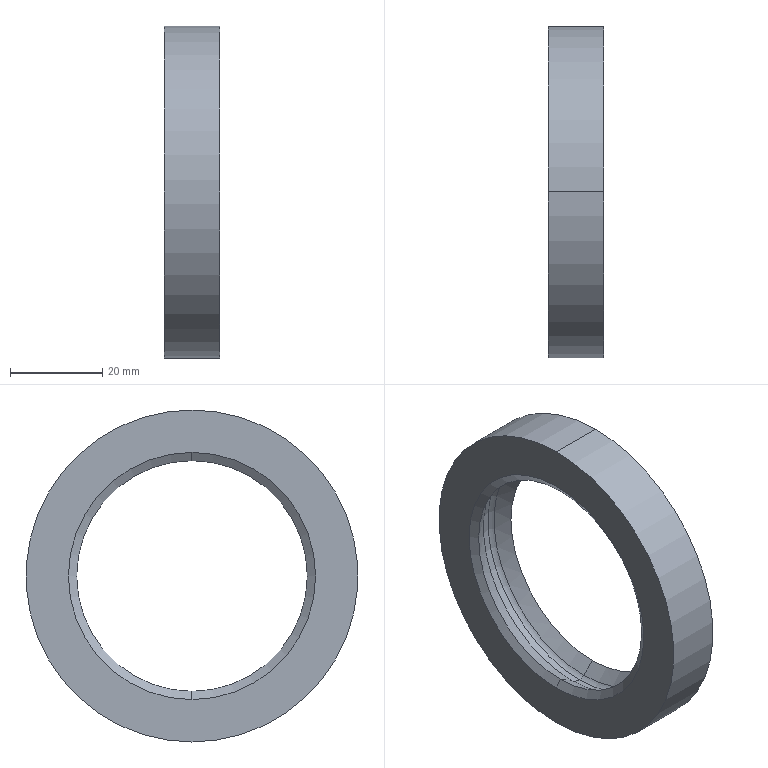Part | STEP file | AMFF-P5-A70-d50-D72-T12 oil seal | 1 solid | 17 faces | box 12 x 72 x 72 mm | volume 22091 mm3 | cone 10 | plane 3 | torus 2 | cylinder 2 | commonest cylinder face diameters 72 x2
STEP:
#1=CARTESIAN_POINT('',(0.,0.,0.));
#2=DIRECTION('',(0.,0.,1.));
#3=DIRECTION('',(1.,0.,0.));
#4=AXIS2_PLACEMENT_3D('',#1,#2,#3);
#5=CARTESIAN_POINT('',(-4.86,0.,25.));
#6=VERTEX_POINT('',#5);
#7=CARTESIAN_POINT('',(-6.,0.,26.8));
#8=VERTEX_POINT('',#7);
#9=CARTESIAN_POINT('',(-6.,0.,26.8));
#10=DIRECTION('',(-0.5351,0.,0.8448));
#11=VECTOR('',#10,1.);
#12=LINE('',#9,#11);
#13=CARTESIAN_POINT('',(-6.,0.,0.));
#14=DIRECTION('',(-1.,0.,0.));
#15=DIRECTION('',(0.,0.,1.));
#16=AXIS2_PLACEMENT_3D('',#13,#14,#15);
#17=CONICAL_SURFACE('',#16,26.8,1.006);
#18=CARTESIAN_POINT('',(6.283,0.));
#19=DIRECTION('',(0.,1.));
#20=VECTOR('',#19,1.);
#21=LINE('',#18,#20);
#22=(GEOMETRIC_REPRESENTATION_CONTEXT(2)PARAMETRIC_REPRESENTATION_CONTEXT()REPRESENTATION_CONTEXT('',''));
#23=DEFINITIONAL_REPRESENTATION('',(#21),#22);
#24=PCURVE('',#17,#23);
#25=CARTESIAN_POINT('',(-6.,0.,0.));
#26=DIRECTION('',(-1.,0.,0.));
#27=DIRECTION('',(0.,0.,1.));
#28=AXIS2_PLACEMENT_3D('',#25,#26,#27);
#29=CONICAL_SURFACE('',#28,26.8,1.006);
#30=CARTESIAN_POINT('',(0.,0.));
#31=DIRECTION('',(0.,1.));
#32=VECTOR('',#31,1.);
#33=LINE('',#30,#32);
#34=(GEOMETRIC_REPRESENTATION_CONTEXT(2)PARAMETRIC_REPRESENTATION_CONTEXT()REPRESENTATION_CONTEXT('',''));
#35=DEFINITIONAL_REPRESENTATION('',(#33),#34);
#36=PCURVE('',#29,#35);
#37=SURFACE_CURVE('',#12,(#24,#36),.PCURVE_S1.);
#38=EDGE_CURVE('',#6,#8,#37,.T.);
#39=ORIENTED_EDGE('',*,*,#38,.T.);
#40=CARTESIAN_POINT('',(-6.,0.,-26.8));
#41=VERTEX_POINT('',#40);
#42=CARTESIAN_POINT('',(-6.,0.,0.));
#43=DIRECTION('',(-1.,0.,0.));
#44=DIRECTION('',(0.,0.,1.));
#45=AXIS2_PLACEMENT_3D('',#42,#43,#44);
#46=CIRCLE('',#45,26.8);
#47=CARTESIAN_POINT('',(0.,0.));
#48=DIRECTION('',(1.,0.));
#49=VECTOR('',#48,1.);
#50=LINE('',#47,#49);
#51=(GEOMETRIC_REPRESENTATION_CONTEXT(2)PARAMETRIC_REPRESENTATION_CONTEXT()REPRESENTATION_CONTEXT('',''));
#52=DEFINITIONAL_REPRESENTATION('',(#50),#51);
#53=PCURVE('',#17,#52);
#54=CARTESIAN_POINT('',(-6.,26.8,0.));
#55=DIRECTION('',(1.,0.,0.));
#56=DIRECTION('',(0.,0.,-1.));
#57=AXIS2_PLACEMENT_3D('',#54,#55,#56);
#58=PLANE('',#57);
#59=CARTESIAN_POINT('',(-26.8,-26.8));
#60=CARTESIAN_POINT('',(-26.8,19.619));
#61=CARTESIAN_POINT('',(13.4,-3.591));
#62=CARTESIAN_POINT('',(53.6,-26.8));
#63=CARTESIAN_POINT('',(13.4,-50.009));
#64=CARTESIAN_POINT('',(-26.8,-73.219));
#65=CARTESIAN_POINT('',(-26.8,-26.8));
#66=(BOUNDED_CURVE()B_SPLINE_CURVE(2,(#59,#60,#61,#62,#63,#64,#65),.UNSPECIFIED.,.T.,.F.)B_SPLINE_CURVE_WITH_KNOTS((1,2,2,2,2,1),(-2.094,0.,2.094,4.189,6.283,8.378),.UNSPECIFIED.)CURVE()GEOMETRIC_REPRESENTATION_ITEM()RATIONAL_B_SPLINE_CURVE((1.,0.5,1.,0.5,1.,0.5,1.))REPRESENTATION_ITEM(''));
#67=(GEOMETRIC_REPRESENTATION_CONTEXT(2)PARAMETRIC_REPRESENTATION_CONTEXT()REPRESENTATION_CONTEXT('',''));
#68=DEFINITIONAL_REPRESENTATION('',(#66),#67);
#69=PCURVE('',#58,#68);
#70=SURFACE_CURVE('',#46,(#53,#69),.PCURVE_S1.);
#71=EDGE_CURVE('',#41,#8,#70,.T.);
#72=ORIENTED_EDGE('',*,*,#71,.F.);
#73=CARTESIAN_POINT('',(-4.86,0.,-25.));
#74=VERTEX_POINT('',#73);
#75=CARTESIAN_POINT('',(-6.,0.,-26.8));
#76=DIRECTION('',(-0.5351,0.,-0.8448));
#77=VECTOR('',#76,1.);
#78=LINE('',#75,#77);
#79=CARTESIAN_POINT('',(3.142,0.));
#80=DIRECTION('',(0.,1.));
#81=VECTOR('',#80,1.);
#82=LINE('',#79,#81);
#83=(GEOMETRIC_REPRESENTATION_CONTEXT(2)PARAMETRIC_REPRESENTATION_CONTEXT()REPRESENTATION_CONTEXT('',''));
#84=DEFINITIONAL_REPRESENTATION('',(#82),#83);
#85=PCURVE('',#17,#84);
#86=CARTESIAN_POINT('',(3.142,0.));
#87=DIRECTION('',(0.,1.));
#88=VECTOR('',#87,1.);
#89=LINE('',#86,#88);
#90=(GEOMETRIC_REPRESENTATION_CONTEXT(2)PARAMETRIC_REPRESENTATION_CONTEXT()REPRESENTATION_CONTEXT('',''));
#91=DEFINITIONAL_REPRESENTATION('',(#89),#90);
#92=PCURVE('',#29,#91);
#93=SURFACE_CURVE('',#78,(#85,#92),.PCURVE_S1.);
#94=EDGE_CURVE('',#74,#41,#93,.T.);
#95=ORIENTED_EDGE('',*,*,#94,.F.);
#96=CARTESIAN_POINT('',(-4.86,0.,0.));
#97=DIRECTION('',(-1.,0.,0.));
#98=DIRECTION('',(0.,0.,1.));
#99=AXIS2_PLACEMENT_3D('',#96,#97,#98);
#100=CIRCLE('',#99,25.);
#101=CARTESIAN_POINT('',(0.,-1.14));
#102=DIRECTION('',(1.,0.));
#103=VECTOR('',#102,1.);
#104=LINE('',#101,#103);
#105=(GEOMETRIC_REPRESENTATION_CONTEXT(2)PARAMETRIC_REPRESENTATION_CONTEXT()REPRESENTATION_CONTEXT('',''));
#106=DEFINITIONAL_REPRESENTATION('',(#104),#105);
#107=PCURVE('',#17,#106);
#108=CARTESIAN_POINT('',(-4.86,0.,0.));
#109=DIRECTION('',(1.,0.,0.));
#110=DIRECTION('',(0.,0.,-1.));
#111=AXIS2_PLACEMENT_3D('',#108,#109,#110);
#112=CONICAL_SURFACE('',#111,25.,0.5404);
#113=CARTESIAN_POINT('',(9.425,0.));
#114=DIRECTION('',(-1.,0.));
#115=VECTOR('',#114,1.);
#116=LINE('',#113,#115);
#117=(GEOMETRIC_REPRESENTATION_CONTEXT(2)PARAMETRIC_REPRESENTATION_CONTEXT()REPRESENTATION_CONTEXT('',''));
#118=DEFINITIONAL_REPRESENTATION('',(#116),#117);
#119=PCURVE('',#112,#118);
#120=SURFACE_CURVE('',#100,(#107,#119),.PCURVE_S1.);
#121=EDGE_CURVE('',#74,#6,#120,.T.);
#122=ORIENTED_EDGE('',*,*,#121,.T.);
#123=EDGE_LOOP('',(#39,#72,#95,#122));
#124=FACE_BOUND('',#123,.F.);
#125=ADVANCED_FACE('',(#124),#17,.F.);
#126=CARTESIAN_POINT('',(-1.26,0.,-27.16));
#127=VERTEX_POINT('',#126);
#128=CARTESIAN_POINT('',(-4.86,0.,-25.));
#129=DIRECTION('',(0.8575,0.,-0.5145));
#130=VECTOR('',#129,1.);
#131=LINE('',#128,#130);
#132=CARTESIAN_POINT('',(6.283,0.));
#133=DIRECTION('',(0.,1.));
#134=VECTOR('',#133,1.);
#135=LINE('',#132,#134);
#136=(GEOMETRIC_REPRESENTATION_CONTEXT(2)PARAMETRIC_REPRESENTATION_CONTEXT()REPRESENTATION_CONTEXT('',''));
#137=DEFINITIONAL_REPRESENTATION('',(#135),#136);
#138=PCURVE('',#112,#137);
#139=CARTESIAN_POINT('',(-4.86,0.,0.));
#140=DIRECTION('',(1.,0.,0.));
#141=DIRECTION('',(0.,0.,-1.));
#142=AXIS2_PLACEMENT_3D('',#139,#140,#141);
#143=CONICAL_SURFACE('',#142,25.,0.5404);
#144=CARTESIAN_POINT('',(0.,0.));
#145=DIRECTION('',(0.,1.));
#146=VECTOR('',#145,1.);
#147=LINE('',#144,#146);
#148=(GEOMETRIC_REPRESENTATION_CONTEXT(2)PARAMETRIC_REPRESENTATION_CONTEXT()REPRESENTATION_CONTEXT('',''));
#149=DEFINITIONAL_REPRESENTATION('',(#147),#148);
#150=PCURVE('',#143,#149);
#151=SURFACE_CURVE('',#131,(#138,#150),.PCURVE_S1.);
#152=EDGE_CURVE('',#74,#127,#151,.T.);
#153=ORIENTED_EDGE('',*,*,#152,.T.);
#154=CARTESIAN_POINT('',(-1.26,0.,27.16));
#155=VERTEX_POINT('',#154);
#156=CARTESIAN_POINT('',(-1.26,0.,0.));
#157=DIRECTION('',(-1.,0.,0.));
#158=DIRECTION('',(0.,0.,1.));
#159=AXIS2_PLACEMENT_3D('',#156,#157,#158);
#160=CIRCLE('',#159,27.16);
#161=CARTESIAN_POINT('',(9.425,3.6));
#162=DIRECTION('',(-1.,0.));
#163=VECTOR('',#162,1.);
#164=LINE('',#161,#163);
#165=(GEOMETRIC_REPRESENTATION_CONTEXT(2)PARAMETRIC_REPRESENTATION_CONTEXT()REPRESENTATION_CONTEXT('',''));
#166=DEFINITIONAL_REPRESENTATION('',(#164),#165);
#167=PCURVE('',#112,#166);
#168=CARTESIAN_POINT('',(-1.26,27.52,0.));
#169=DIRECTION('',(-1.,0.,0.));
#170=DIRECTION('',(0.,0.,1.));
#171=AXIS2_PLACEMENT_3D('',#168,#169,#170);
#172=PLANE('',#171);
#173=CARTESIAN_POINT('',(0.,-27.52));
#174=DIRECTION('',(1.,0.));
#175=AXIS2_PLACEMENT_2D('',#173,#174);
#176=CIRCLE('',#175,27.16);
#177=(GEOMETRIC_REPRESENTATION_CONTEXT(2)PARAMETRIC_REPRESENTATION_CONTEXT()REPRESENTATION_CONTEXT('',''));
#178=DEFINITIONAL_REPRESENTATION('',(#176),#177);
#179=PCURVE('',#172,#178);
#180=SURFACE_CURVE('',#160,(#167,#179),.PCURVE_S1.);
#181=EDGE_CURVE('',#127,#155,#180,.T.);
#182=ORIENTED_EDGE('',*,*,#181,.T.);
#183=CARTESIAN_POINT('',(-4.86,0.,25.));
#184=DIRECTION('',(0.8575,0.,0.5145));
#185=VECTOR('',#184,1.);
#186=LINE('',#183,#185);
#187=CARTESIAN_POINT('',(3.142,0.));
#188=DIRECTION('',(0.,1.));
#189=VECTOR('',#188,1.);
#190=LINE('',#187,#189);
#191=(GEOMETRIC_REPRESENTATION_CONTEXT(2)PARAMETRIC_REPRESENTATION_CONTEXT()REPRESENTATION_CONTEXT('',''));
#192=DEFINITIONAL_REPRESENTATION('',(#190),#191);
#193=PCURVE('',#112,#192);
#194=CARTESIAN_POINT('',(3.142,0.));
#195=DIRECTION('',(0.,1.));
#196=VECTOR('',#195,1.);
#197=LINE('',#194,#196);
#198=(GEOMETRIC_REPRESENTATION_CONTEXT(2)PARAMETRIC_REPRESENTATION_CONTEXT()REPRESENTATION_CONTEXT('',''));
#199=DEFINITIONAL_REPRESENTATION('',(#197),#198);
#200=PCURVE('',#143,#199);
#201=SURFACE_CURVE('',#186,(#193,#200),.PCURVE_S1.);
#202=EDGE_CURVE('',#6,#155,#201,.T.);
#203=ORIENTED_EDGE('',*,*,#202,.F.);
#204=ORIENTED_EDGE('',*,*,#121,.F.);
#205=EDGE_LOOP('',(#153,#182,#203,#204));
#206=FACE_BOUND('',#205,.F.);
#207=ADVANCED_FACE('',(#206),#112,.F.);
#208=CARTESIAN_POINT('',(-1.26,0.,-27.52));
#209=VERTEX_POINT('',#208);
#210=CARTESIAN_POINT('',(1.14,0.,-28.191));
#211=VERTEX_POINT('',#210);
#212=CARTESIAN_POINT('',(-1.26,0.,-27.52));
#213=DIRECTION('',(0.9631,0.,-0.2693));
#214=VECTOR('',#213,1.);
#215=LINE('',#212,#214);
#216=CARTESIAN_POINT('',(-1.26,0.,0.));
#217=DIRECTION('',(1.,0.,0.));
#218=DIRECTION('',(0.,0.,-1.));
#219=AXIS2_PLACEMENT_3D('',#216,#217,#218);
#220=CONICAL_SURFACE('',#219,27.52,0.2727);
#221=CARTESIAN_POINT('',(6.283,0.));
#222=DIRECTION('',(0.,1.));
#223=VECTOR('',#222,1.);
#224=LINE('',#221,#223);
#225=(GEOMETRIC_REPRESENTATION_CONTEXT(2)PARAMETRIC_REPRESENTATION_CONTEXT()REPRESENTATION_CONTEXT('',''));
#226=DEFINITIONAL_REPRESENTATION('',(#224),#225);
#227=PCURVE('',#220,#226);
#228=CARTESIAN_POINT('',(-1.26,0.,0.));
#229=DIRECTION('',(1.,0.,0.));
#230=DIRECTION('',(0.,0.,-1.));
#231=AXIS2_PLACEMENT_3D('',#228,#229,#230);
#232=CONICAL_SURFACE('',#231,27.52,0.2727);
#233=CARTESIAN_POINT('',(0.,0.));
#234=DIRECTION('',(0.,1.));
#235=VECTOR('',#234,1.);
#236=LINE('',#233,#235);
#237=(GEOMETRIC_REPRESENTATION_CONTEXT(2)PARAMETRIC_REPRESENTATION_CONTEXT()REPRESENTATION_CONTEXT('',''));
#238=DEFINITIONAL_REPRESENTATION('',(#236),#237);
#239=PCURVE('',#232,#238);
#240=SURFACE_CURVE('',#215,(#227,#239),.PCURVE_S1.);
#241=EDGE_CURVE('',#209,#211,#240,.T.);
#242=ORIENTED_EDGE('',*,*,#241,.T.);
#243=CARTESIAN_POINT('',(1.14,0.,28.191));
#244=VERTEX_POINT('',#243);
#245=CARTESIAN_POINT('',(1.14,0.,0.));
#246=DIRECTION('',(-1.,0.,0.));
#247=DIRECTION('',(0.,0.,1.));
#248=AXIS2_PLACEMENT_3D('',#245,#246,#247);
#249=CIRCLE('',#248,28.191);
#250=CARTESIAN_POINT('',(9.425,2.4));
#251=DIRECTION('',(-1.,0.));
#252=VECTOR('',#251,1.);
#253=LINE('',#250,#252);
#254=(GEOMETRIC_REPRESENTATION_CONTEXT(2)PARAMETRIC_REPRESENTATION_CONTEXT()REPRESENTATION_CONTEXT('',''));
#255=DEFINITIONAL_REPRESENTATION('',(#253),#254);
#256=PCURVE('',#220,#255);
#257=CARTESIAN_POINT('',(0.3749,0.,0.));
#258=DIRECTION('',(-1.,0.,0.));
#259=DIRECTION('',(0.,0.,1.));
#260=AXIS2_PLACEMENT_3D('',#257,#258,#259);
#261=TOROIDAL_SURFACE('',#260,25.415,2.88);
#262=CARTESIAN_POINT('',(0.,6.014));
#263=DIRECTION('',(1.,0.));
#264=VECTOR('',#263,1.);
#265=LINE('',#262,#264);
#266=(GEOMETRIC_REPRESENTATION_CONTEXT(2)PARAMETRIC_REPRESENTATION_CONTEXT()REPRESENTATION_CONTEXT('',''));
#267=DEFINITIONAL_REPRESENTATION('',(#265),#266);
#268=PCURVE('',#261,#267);
#269=SURFACE_CURVE('',#249,(#256,#268),.PCURVE_S1.);
#270=EDGE_CURVE('',#211,#244,#269,.T.);
#271=ORIENTED_EDGE('',*,*,#270,.T.);
#272=CARTESIAN_POINT('',(-1.26,0.,27.52));
#273=VERTEX_POINT('',#272);
#274=CARTESIAN_POINT('',(-1.26,0.,27.52));
#275=DIRECTION('',(0.9631,0.,0.2693));
#276=VECTOR('',#275,1.);
#277=LINE('',#274,#276);
#278=CARTESIAN_POINT('',(3.142,0.));
#279=DIRECTION('',(0.,1.));
#280=VECTOR('',#279,1.);
#281=LINE('',#278,#280);
#282=(GEOMETRIC_REPRESENTATION_CONTEXT(2)PARAMETRIC_REPRESENTATION_CONTEXT()REPRESENTATION_CONTEXT('',''));
#283=DEFINITIONAL_REPRESENTATION('',(#281),#282);
#284=PCURVE('',#220,#283);
#285=CARTESIAN_POINT('',(3.142,0.));
#286=DIRECTION('',(0.,1.));
#287=VECTOR('',#286,1.);
#288=LINE('',#285,#287);
#289=(GEOMETRIC_REPRESENTATION_CONTEXT(2)PARAMETRIC_REPRESENTATION_CONTEXT()REPRESENTATION_CONTEXT('',''));
#290=DEFINITIONAL_REPRESENTATION('',(#288),#289);
#291=PCURVE('',#232,#290);
#292=SURFACE_CURVE('',#277,(#284,#291),.PCURVE_S1.);
#293=EDGE_CURVE('',#273,#244,#292,.T.);
#294=ORIENTED_EDGE('',*,*,#293,.F.);
#295=CARTESIAN_POINT('',(-1.26,0.,0.));
#296=DIRECTION('',(-1.,0.,0.));
#297=DIRECTION('',(0.,0.,1.));
#298=AXIS2_PLACEMENT_3D('',#295,#296,#297);
#299=CIRCLE('',#298,27.52);
#300=CARTESIAN_POINT('',(9.425,0.));
#301=DIRECTION('',(-1.,0.));
#302=VECTOR('',#301,1.);
#303=LINE('',#300,#302);
#304=(GEOMETRIC_REPRESENTATION_CONTEXT(2)PARAMETRIC_REPRESENTATION_CONTEXT()REPRESENTATION_CONTEXT('',''));
#305=DEFINITIONAL_REPRESENTATION('',(#303),#304);
#306=PCURVE('',#220,#305);
#307=CARTESIAN_POINT('',(0.,-27.52));
#308=DIRECTION('',(1.,0.));
#309=AXIS2_PLACEMENT_2D('',#307,#308);
#310=CIRCLE('',#309,27.52);
#311=(GEOMETRIC_REPRESENTATION_CONTEXT(2)PARAMETRIC_REPRESENTATION_CONTEXT()REPRESENTATION_CONTEXT('',''));
#312=DEFINITIONAL_REPRESENTATION('',(#310),#311);
#313=PCURVE('',#172,#312);
#314=SURFACE_CURVE('',#299,(#306,#313),.PCURVE_S1.);
#315=EDGE_CURVE('',#209,#273,#314,.T.);
#316=ORIENTED_EDGE('',*,*,#315,.F.);
#317=EDGE_LOOP('',(#242,#271,#294,#316));
#318=FACE_BOUND('',#317,.F.);
#319=ADVANCED_FACE('',(#318),#220,.F.);
#320=CARTESIAN_POINT('',(2.34,0.,27.52));
#321=VERTEX_POINT('',#320);
#322=CARTESIAN_POINT('',(0.3749,0.,25.415));
#323=DIRECTION('',(0.,-1.,0.));
#324=DIRECTION('',(0.,0.,-1.));
#325=AXIS2_PLACEMENT_3D('',#322,#323,#324);
#326=CIRCLE('',#325,2.88);
#327=CARTESIAN_POINT('',(6.283,3.142));
#328=DIRECTION('',(0.,1.));
#329=VECTOR('',#328,1.);
#330=LINE('',#327,#329);
#331=(GEOMETRIC_REPRESENTATION_CONTEXT(2)PARAMETRIC_REPRESENTATION_CONTEXT()REPRESENTATION_CONTEXT('',''));
#332=DEFINITIONAL_REPRESENTATION('',(#330),#331);
#333=PCURVE('',#261,#332);
#334=CARTESIAN_POINT('',(0.3749,0.,0.));
#335=DIRECTION('',(-1.,0.,0.));
#336=DIRECTION('',(0.,0.,1.));
#337=AXIS2_PLACEMENT_3D('',#334,#335,#336);
#338=TOROIDAL_SURFACE('',#337,25.415,2.88);
#339=CARTESIAN_POINT('',(0.,3.142));
#340=DIRECTION('',(0.,1.));
#341=VECTOR('',#340,1.);
#342=LINE('',#339,#341);
#343=(GEOMETRIC_REPRESENTATION_CONTEXT(2)PARAMETRIC_REPRESENTATION_CONTEXT()REPRESENTATION_CONTEXT('',''));
#344=DEFINITIONAL_REPRESENTATION('',(#342),#343);
#345=PCURVE('',#338,#344);
#346=SURFACE_CURVE('',#326,(#333,#345),.PCURVE_S1.);
#347=EDGE_CURVE('',#321,#244,#346,.T.);
#348=ORIENTED_EDGE('',*,*,#347,.T.);
#349=ORIENTED_EDGE('',*,*,#270,.F.);
#350=CARTESIAN_POINT('',(2.34,0.,-27.52));
#351=VERTEX_POINT('',#350);
#352=CARTESIAN_POINT('',(0.3749,0.,-25.415));
#353=DIRECTION('',(0.,1.,0.));
#354=DIRECTION('',(0.,0.,1.));
#355=AXIS2_PLACEMENT_3D('',#352,#353,#354);
#356=CIRCLE('',#355,2.88);
#357=CARTESIAN_POINT('',(3.142,3.142));
#358=DIRECTION('',(0.,1.));
#359=VECTOR('',#358,1.);
#360=LINE('',#357,#359);
#361=(GEOMETRIC_REPRESENTATION_CONTEXT(2)PARAMETRIC_REPRESENTATION_CONTEXT()REPRESENTATION_CONTEXT('',''));
#362=DEFINITIONAL_REPRESENTATION('',(#360),#361);
#363=PCURVE('',#261,#362);
#364=CARTESIAN_POINT('',(3.142,3.142));
#365=DIRECTION('',(0.,1.));
#366=VECTOR('',#365,1.);
#367=LINE('',#364,#366);
#368=(GEOMETRIC_REPRESENTATION_CONTEXT(2)PARAMETRIC_REPRESENTATION_CONTEXT()REPRESENTATION_CONTEXT('',''));
#369=DEFINITIONAL_REPRESENTATION('',(#367),#368);
#370=PCURVE('',#338,#369);
#371=SURFACE_CURVE('',#356,(#363,#370),.PCURVE_S1.);
#372=EDGE_CURVE('',#351,#211,#371,.T.);
#373=ORIENTED_EDGE('',*,*,#372,.F.);
#374=CARTESIAN_POINT('',(2.34,0.,0.));
#375=DIRECTION('',(-1.,0.,0.));
#376=DIRECTION('',(0.,0.,1.));
#377=AXIS2_PLACEMENT_3D('',#374,#375,#376);
#378=CIRCLE('',#377,27.52);
#379=CARTESIAN_POINT('',(0.,5.532));
#380=DIRECTION('',(1.,0.));
#381=VECTOR('',#380,1.);
#382=LINE('',#379,#381);
#383=(GEOMETRIC_REPRESENTATION_CONTEXT(2)PARAMETRIC_REPRESENTATION_CONTEXT()REPRESENTATION_CONTEXT('',''));
#384=DEFINITIONAL_REPRESENTATION('',(#382),#383);
#385=PCURVE('',#261,#384);
#386=CARTESIAN_POINT('',(2.34,0.,0.));
#387=DIRECTION('',(-1.,0.,0.));
#388=DIRECTION('',(0.,0.,1.));
#389=AXIS2_PLACEMENT_3D('',#386,#387,#388);
#390=CONICAL_SURFACE('',#389,27.52,0.7509);
#391=CARTESIAN_POINT('',(0.,0.));
#392=DIRECTION('',(1.,0.));
#393=VECTOR('',#392,1.);
#394=LINE('',#391,#393);
#395=(GEOMETRIC_REPRESENTATION_CONTEXT(2)PARAMETRIC_REPRESENTATION_CONTEXT()REPRESENTATION_CONTEXT('',''));
#396=DEFINITIONAL_REPRESENTATION('',(#394),#395);
#397=PCURVE('',#390,#396);
#398=SURFACE_CURVE('',#378,(#385,#397),.PCURVE_S1.);
#399=EDGE_CURVE('',#351,#321,#398,.T.);
#400=ORIENTED_EDGE('',*,*,#399,.T.);
#401=EDGE_LOOP('',(#348,#349,#373,#400));
#402=FACE_BOUND('',#401,.F.);
#403=ADVANCED_FACE('',(#402),#261,.F.);
#404=CARTESIAN_POINT('',(5.04,0.,25.));
#405=VERTEX_POINT('',#404);
#406=CARTESIAN_POINT('',(2.34,0.,27.52));
#407=DIRECTION('',(-0.7311,0.,0.6823));
#408=VECTOR('',#407,1.);
#409=LINE('',#406,#408);
#410=CARTESIAN_POINT('',(6.283,0.));
#411=DIRECTION('',(0.,1.));
#412=VECTOR('',#411,1.);
#413=LINE('',#410,#412);
#414=(GEOMETRIC_REPRESENTATION_CONTEXT(2)PARAMETRIC_REPRESENTATION_CONTEXT()REPRESENTATION_CONTEXT('',''));
#415=DEFINITIONAL_REPRESENTATION('',(#413),#414);
#416=PCURVE('',#390,#415);
#417=CARTESIAN_POINT('',(2.34,0.,0.));
#418=DIRECTION('',(-1.,0.,0.));
#419=DIRECTION('',(0.,0.,1.));
#420=AXIS2_PLACEMENT_3D('',#417,#418,#419);
#421=CONICAL_SURFACE('',#420,27.52,0.7509);
#422=CARTESIAN_POINT('',(0.,0.));
#423=DIRECTION('',(0.,1.));
#424=VECTOR('',#423,1.);
#425=LINE('',#422,#424);
#426=(GEOMETRIC_REPRESENTATION_CONTEXT(2)PARAMETRIC_REPRESENTATION_CONTEXT()REPRESENTATION_CONTEXT('',''));
#427=DEFINITIONAL_REPRESENTATION('',(#425),#426);
#428=PCURVE('',#421,#427);
#429=SURFACE_CURVE('',#409,(#416,#428),.PCURVE_S1.);
#430=EDGE_CURVE('',#405,#321,#429,.T.);
#431=ORIENTED_EDGE('',*,*,#430,.T.);
#432=ORIENTED_EDGE('',*,*,#399,.F.);
#433=CARTESIAN_POINT('',(5.04,0.,-25.));
#434=VERTEX_POINT('',#433);
#435=CARTESIAN_POINT('',(2.34,0.,-27.52));
#436=DIRECTION('',(-0.7311,0.,-0.6823));
#437=VECTOR('',#436,1.);
#438=LINE('',#435,#437);
#439=CARTESIAN_POINT('',(3.142,0.));
#440=DIRECTION('',(0.,1.));
#441=VECTOR('',#440,1.);
#442=LINE('',#439,#441);
#443=(GEOMETRIC_REPRESENTATION_CONTEXT(2)PARAMETRIC_REPRESENTATION_CONTEXT()REPRESENTATION_CONTEXT('',''));
#444=DEFINITIONAL_REPRESENTATION('',(#442),#443);
#445=PCURVE('',#390,#444);
#446=CARTESIAN_POINT('',(3.142,0.));
#447=DIRECTION('',(0.,1.));
#448=VECTOR('',#447,1.);
#449=LINE('',#446,#448);
#450=(GEOMETRIC_REPRESENTATION_CONTEXT(2)PARAMETRIC_REPRESENTATION_CONTEXT()REPRESENTATION_CONTEXT('',''));
#451=DEFINITIONAL_REPRESENTATION('',(#449),#450);
#452=PCURVE('',#421,#451);
#453=SURFACE_CURVE('',#438,(#445,#452),.PCURVE_S1.);
#454=EDGE_CURVE('',#434,#351,#453,.T.);
#455=ORIENTED_EDGE('',*,*,#454,.F.);
#456=CARTESIAN_POINT('',(5.04,0.,0.));
#457=DIRECTION('',(-1.,0.,0.));
#458=DIRECTION('',(0.,0.,1.));
#459=AXIS2_PLACEMENT_3D('',#456,#457,#458);
#460=CIRCLE('',#459,25.);
#461=CARTESIAN_POINT('',(0.,-2.7));
#462=DIRECTION('',(1.,0.));
#463=VECTOR('',#462,1.);
#464=LINE('',#461,#463);
#465=(GEOMETRIC_REPRESENTATION_CONTEXT(2)PARAMETRIC_REPRESENTATION_CONTEXT()REPRESENTATION_CONTEXT('',''));
#466=DEFINITIONAL_REPRESENTATION('',(#464),#465);
#467=PCURVE('',#390,#466);
#468=CARTESIAN_POINT('',(5.04,0.,0.));
#469=DIRECTION('',(1.,0.,0.));
#470=DIRECTION('',(0.,0.,-1.));
#471=AXIS2_PLACEMENT_3D('',#468,#469,#470);
#472=CONICAL_SURFACE('',#471,25.,1.081);
#473=CARTESIAN_POINT('',(9.425,0.));
#474=DIRECTION('',(-1.,0.));
#475=VECTOR('',#474,1.);
#476=LINE('',#473,#475);
#477=(GEOMETRIC_REPRESENTATION_CONTEXT(2)PARAMETRIC_REPRESENTATION_CONTEXT()REPRESENTATION_CONTEXT('',''));
#478=DEFINITIONAL_REPRESENTATION('',(#476),#477);
#479=PCURVE('',#472,#478);
#480=SURFACE_CURVE('',#460,(#467,#479),.PCURVE_S1.);
#481=EDGE_CURVE('',#434,#405,#480,.T.);
#482=ORIENTED_EDGE('',*,*,#481,.T.);
#483=EDGE_LOOP('',(#431,#432,#455,#482));
#484=FACE_BOUND('',#483,.F.);
#485=ADVANCED_FACE('',(#484),#390,.F.);
#486=CARTESIAN_POINT('',(6.,0.,-26.8));
#487=VERTEX_POINT('',#486);
#488=CARTESIAN_POINT('',(5.04,0.,-25.));
#489=DIRECTION('',(0.4706,0.,-0.8824));
#490=VECTOR('',#489,1.);
#491=LINE('',#488,#490);
#492=CARTESIAN_POINT('',(6.283,0.));
#493=DIRECTION('',(0.,1.));
#494=VECTOR('',#493,1.);
#495=LINE('',#492,#494);
#496=(GEOMETRIC_REPRESENTATION_CONTEXT(2)PARAMETRIC_REPRESENTATION_CONTEXT()REPRESENTATION_CONTEXT('',''));
#497=DEFINITIONAL_REPRESENTATION('',(#495),#496);
#498=PCURVE('',#472,#497);
#499=CARTESIAN_POINT('',(5.04,0.,0.));
#500=DIRECTION('',(1.,0.,0.));
#501=DIRECTION('',(0.,0.,-1.));
#502=AXIS2_PLACEMENT_3D('',#499,#500,#501);
#503=CONICAL_SURFACE('',#502,25.,1.081);
#504=CARTESIAN_POINT('',(0.,0.));
#505=DIRECTION('',(0.,1.));
#506=VECTOR('',#505,1.);
#507=LINE('',#504,#506);
#508=(GEOMETRIC_REPRESENTATION_CONTEXT(2)PARAMETRIC_REPRESENTATION_CONTEXT()REPRESENTATION_CONTEXT('',''));
#509=DEFINITIONAL_REPRESENTATION('',(#507),#508);
#510=PCURVE('',#503,#509);
#511=SURFACE_CURVE('',#491,(#498,#510),.PCURVE_S1.);
#512=EDGE_CURVE('',#434,#487,#511,.T.);
#513=ORIENTED_EDGE('',*,*,#512,.T.);
#514=CARTESIAN_POINT('',(6.,0.,26.8));
#515=VERTEX_POINT('',#514);
#516=CARTESIAN_POINT('',(6.,0.,0.));
#517=DIRECTION('',(-1.,0.,0.));
#518=DIRECTION('',(0.,0.,1.));
#519=AXIS2_PLACEMENT_3D('',#516,#517,#518);
#520=CIRCLE('',#519,26.8);
#521=CARTESIAN_POINT('',(9.425,0.96));
#522=DIRECTION('',(-1.,0.));
#523=VECTOR('',#522,1.);
#524=LINE('',#521,#523);
#525=(GEOMETRIC_REPRESENTATION_CONTEXT(2)PARAMETRIC_REPRESENTATION_CONTEXT()REPRESENTATION_CONTEXT('',''));
#526=DEFINITIONAL_REPRESENTATION('',(#524),#525);
#527=PCURVE('',#472,#526);
#528=CARTESIAN_POINT('',(6.,26.8,0.));
#529=DIRECTION('',(-1.,0.,0.));
#530=DIRECTION('',(0.,0.,1.));
#531=AXIS2_PLACEMENT_3D('',#528,#529,#530);
#532=PLANE('',#531);
#533=CARTESIAN_POINT('',(0.,-26.8));
#534=DIRECTION('',(1.,0.));
#535=AXIS2_PLACEMENT_2D('',#533,#534);
#536=CIRCLE('',#535,26.8);
#537=(GEOMETRIC_REPRESENTATION_CONTEXT(2)PARAMETRIC_REPRESENTATION_CONTEXT()REPRESENTATION_CONTEXT('',''));
#538=DEFINITIONAL_REPRESENTATION('',(#536),#537);
#539=PCURVE('',#532,#538);
#540=SURFACE_CURVE('',#520,(#527,#539),.PCURVE_S1.);
#541=EDGE_CURVE('',#487,#515,#540,.T.);
#542=ORIENTED_EDGE('',*,*,#541,.T.);
#543=CARTESIAN_POINT('',(5.04,0.,25.));
#544=DIRECTION('',(0.4706,0.,0.8824));
#545=VECTOR('',#544,1.);
#546=LINE('',#543,#545);
#547=CARTESIAN_POINT('',(3.142,0.));
#548=DIRECTION('',(0.,1.));
#549=VECTOR('',#548,1.);
#550=LINE('',#547,#549);
#551=(GEOMETRIC_REPRESENTATION_CONTEXT(2)PARAMETRIC_REPRESENTATION_CONTEXT()REPRESENTATION_CONTEXT('',''));
#552=DEFINITIONAL_REPRESENTATION('',(#550),#551);
#553=PCURVE('',#472,#552);
#554=CARTESIAN_POINT('',(3.142,0.));
#555=DIRECTION('',(0.,1.));
#556=VECTOR('',#555,1.);
#557=LINE('',#554,#556);
#558=(GEOMETRIC_REPRESENTATION_CONTEXT(2)PARAMETRIC_REPRESENTATION_CONTEXT()REPRESENTATION_CONTEXT('',''));
#559=DEFINITIONAL_REPRESENTATION('',(#557),#558);
#560=PCURVE('',#503,#559);
#561=SURFACE_CURVE('',#546,(#553,#560),.PCURVE_S1.);
#562=EDGE_CURVE('',#405,#515,#561,.T.);
#563=ORIENTED_EDGE('',*,*,#562,.F.);
#564=ORIENTED_EDGE('',*,*,#481,.F.);
#565=EDGE_LOOP('',(#513,#542,#563,#564));
#566=FACE_BOUND('',#565,.F.);
#567=ADVANCED_FACE('',(#566),#472,.F.);
#568=CARTESIAN_POINT('',(6.,0.,36.));
#569=VERTEX_POINT('',#568);
#570=CARTESIAN_POINT('',(6.,0.,-36.));
#571=VERTEX_POINT('',#570);
#572=CARTESIAN_POINT('',(6.,0.,0.));
#573=DIRECTION('',(-1.,0.,0.));
#574=DIRECTION('',(0.,0.,1.));
#575=AXIS2_PLACEMENT_3D('',#572,#573,#574);
#576=CIRCLE('',#575,36.);
#577=CARTESIAN_POINT('',(-1000.,0.,0.));
#578=DIRECTION('',(-1.,0.,0.));
#579=DIRECTION('',(0.,0.,1.));
#580=AXIS2_PLACEMENT_3D('',#577,#578,#579);
#581=CYLINDRICAL_SURFACE('',#580,36.);
#582=CARTESIAN_POINT('',(0.,-1006.));
#583=DIRECTION('',(1.,0.));
#584=VECTOR('',#583,1.);
#585=LINE('',#582,#584);
#586=(GEOMETRIC_REPRESENTATION_CONTEXT(2)PARAMETRIC_REPRESENTATION_CONTEXT()REPRESENTATION_CONTEXT('',''));
#587=DEFINITIONAL_REPRESENTATION('',(#585),#586);
#588=PCURVE('',#581,#587);
#589=CARTESIAN_POINT('',(0.,-26.8));
#590=DIRECTION('',(1.,0.));
#591=AXIS2_PLACEMENT_2D('',#589,#590);
#592=CIRCLE('',#591,36.);
#593=(GEOMETRIC_REPRESENTATION_CONTEXT(2)PARAMETRIC_REPRESENTATION_CONTEXT()REPRESENTATION_CONTEXT('',''));
#594=DEFINITIONAL_REPRESENTATION('',(#592),#593);
#595=PCURVE('',#532,#594);
#596=SURFACE_CURVE('',#576,(#588,#595),.PCURVE_S1.);
#597=EDGE_CURVE('',#569,#571,#596,.T.);
#598=ORIENTED_EDGE('',*,*,#597,.T.);
#599=CARTESIAN_POINT('',(-6.,0.,-36.));
#600=VERTEX_POINT('',#599);
#601=CARTESIAN_POINT('',(-1000.,0.,-36.));
#602=DIRECTION('',(-1.,0.,0.));
#603=VECTOR('',#602,1.);
#604=LINE('',#601,#603);
#605=CARTESIAN_POINT('',(3.142,0.));
#606=DIRECTION('',(0.,1.));
#607=VECTOR('',#606,1.);
#608=LINE('',#605,#607);
#609=(GEOMETRIC_REPRESENTATION_CONTEXT(2)PARAMETRIC_REPRESENTATION_CONTEXT()REPRESENTATION_CONTEXT('',''));
#610=DEFINITIONAL_REPRESENTATION('',(#608),#609);
#611=PCURVE('',#581,#610);
#612=CARTESIAN_POINT('',(-1000.,0.,0.));
#613=DIRECTION('',(-1.,0.,0.));
#614=DIRECTION('',(0.,0.,1.));
#615=AXIS2_PLACEMENT_3D('',#612,#613,#614);
#616=CYLINDRICAL_SURFACE('',#615,36.);
#617=CARTESIAN_POINT('',(3.142,0.));
#618=DIRECTION('',(0.,1.));
#619=VECTOR('',#618,1.);
#620=LINE('',#617,#619);
#621=(GEOMETRIC_REPRESENTATION_CONTEXT(2)PARAMETRIC_REPRESENTATION_CONTEXT()REPRESENTATION_CONTEXT('',''));
#622=DEFINITIONAL_REPRESENTATION('',(#620),#621);
#623=PCURVE('',#616,#622);
#624=SURFACE_CURVE('',#604,(#611,#623),.PCURVE_S1.);
#625=EDGE_CURVE('',#571,#600,#624,.T.);
#626=ORIENTED_EDGE('',*,*,#625,.T.);
#627=CARTESIAN_POINT('',(-6.,0.,36.));
#628=VERTEX_POINT('',#627);
#629=CARTESIAN_POINT('',(-6.,0.,0.));
#630=DIRECTION('',(-1.,0.,0.));
#631=DIRECTION('',(0.,0.,1.));
#632=AXIS2_PLACEMENT_3D('',#629,#630,#631);
#633=CIRCLE('',#632,36.);
#634=CARTESIAN_POINT('',(0.,-994.));
#635=DIRECTION('',(1.,0.));
#636=VECTOR('',#635,1.);
#637=LINE('',#634,#636);
#638=(GEOMETRIC_REPRESENTATION_CONTEXT(2)PARAMETRIC_REPRESENTATION_CONTEXT()REPRESENTATION_CONTEXT('',''));
#639=DEFINITIONAL_REPRESENTATION('',(#637),#638);
#640=PCURVE('',#581,#639);
#641=CARTESIAN_POINT('',(-36.,-26.8));
#642=CARTESIAN_POINT('',(-36.,35.554));
#643=CARTESIAN_POINT('',(18.,4.377));
#644=CARTESIAN_POINT('',(72.,-26.8));
#645=CARTESIAN_POINT('',(18.,-57.977));
#646=CARTESIAN_POINT('',(-36.,-89.154));
#647=CARTESIAN_POINT('',(-36.,-26.8));
#648=(BOUNDED_CURVE()B_SPLINE_CURVE(2,(#641,#642,#643,#644,#645,#646,#647),.UNSPECIFIED.,.T.,.F.)B_SPLINE_CURVE_WITH_KNOTS((1,2,2,2,2,1),(-2.094,0.,2.094,4.189,6.283,8.378),.UNSPECIFIED.)CURVE()GEOMETRIC_REPRESENTATION_ITEM()RATIONAL_B_SPLINE_CURVE((1.,0.5,1.,0.5,1.,0.5,1.))REPRESENTATION_ITEM(''));
#649=(GEOMETRIC_REPRESENTATION_CONTEXT(2)PARAMETRIC_REPRESENTATION_CONTEXT()REPRESENTATION_CONTEXT('',''));
#650=DEFINITIONAL_REPRESENTATION('',(#648),#649);
#651=PCURVE('',#58,#650);
#652=SURFACE_CURVE('',#633,(#640,#651),.PCURVE_S1.);
#653=EDGE_CURVE('',#628,#600,#652,.T.);
#654=ORIENTED_EDGE('',*,*,#653,.F.);
#655=CARTESIAN_POINT('',(-1000.,0.,36.));
#656=DIRECTION('',(-1.,0.,0.));
#657=VECTOR('',#656,1.);
#658=LINE('',#655,#657);
#659=CARTESIAN_POINT('',(0.,0.));
#660=DIRECTION('',(0.,1.));
#661=VECTOR('',#660,1.);
#662=LINE('',#659,#661);
#663=(GEOMETRIC_REPRESENTATION_CONTEXT(2)PARAMETRIC_REPRESENTATION_CONTEXT()REPRESENTATION_CONTEXT('',''));
#664=DEFINITIONAL_REPRESENTATION('',(#662),#663);
#665=PCURVE('',#581,#664);
#666=CARTESIAN_POINT('',(6.283,0.));
#667=DIRECTION('',(0.,1.));
#668=VECTOR('',#667,1.);
#669=LINE('',#666,#668);
#670=(GEOMETRIC_REPRESENTATION_CONTEXT(2)PARAMETRIC_REPRESENTATION_CONTEXT()REPRESENTATION_CONTEXT('',''));
#671=DEFINITIONAL_REPRESENTATION('',(#669),#670);
#672=PCURVE('',#616,#671);
#673=SURFACE_CURVE('',#658,(#665,#672),.PCURVE_S1.);
#674=EDGE_CURVE('',#569,#628,#673,.T.);
#675=ORIENTED_EDGE('',*,*,#674,.F.);
#676=EDGE_LOOP('',(#598,#626,#654,#675));
#677=FACE_BOUND('',#676,.T.);
#678=ADVANCED_FACE('',(#677),#581,.T.);
#679=CARTESIAN_POINT('',(-6.,0.,0.));
#680=DIRECTION('',(-1.,0.,0.));
#681=DIRECTION('',(0.,0.,1.));
#682=AXIS2_PLACEMENT_3D('',#679,#680,#681);
#683=CIRCLE('',#682,26.8);
#684=CARTESIAN_POINT('',(-26.8,-26.8));
#685=CARTESIAN_POINT('',(-26.8,19.619));
#686=CARTESIAN_POINT('',(13.4,-3.591));
#687=CARTESIAN_POINT('',(53.6,-26.8));
#688=CARTESIAN_POINT('',(13.4,-50.009));
#689=CARTESIAN_POINT('',(-26.8,-73.219));
#690=CARTESIAN_POINT('',(-26.8,-26.8));
#691=(BOUNDED_CURVE()B_SPLINE_CURVE(2,(#684,#685,#686,#687,#688,#689,#690),.UNSPECIFIED.,.T.,.F.)B_SPLINE_CURVE_WITH_KNOTS((1,2,2,2,2,1),(-2.094,0.,2.094,4.189,6.283,8.378),.UNSPECIFIED.)CURVE()GEOMETRIC_REPRESENTATION_ITEM()RATIONAL_B_SPLINE_CURVE((1.,0.5,1.,0.5,1.,0.5,1.))REPRESENTATION_ITEM(''));
#692=(GEOMETRIC_REPRESENTATION_CONTEXT(2)PARAMETRIC_REPRESENTATION_CONTEXT()REPRESENTATION_CONTEXT('',''));
#693=DEFINITIONAL_REPRESENTATION('',(#691),#692);
#694=PCURVE('',#58,#693);
#695=CARTESIAN_POINT('',(0.,0.));
#696=DIRECTION('',(1.,0.));
#697=VECTOR('',#696,1.);
#698=LINE('',#695,#697);
#699=(GEOMETRIC_REPRESENTATION_CONTEXT(2)PARAMETRIC_REPRESENTATION_CONTEXT()REPRESENTATION_CONTEXT('',''));
#700=DEFINITIONAL_REPRESENTATION('',(#698),#699);
#701=PCURVE('',#29,#700);
#702=SURFACE_CURVE('',#683,(#694,#701),.PCURVE_S1.);
#703=EDGE_CURVE('',#8,#41,#702,.T.);
#704=ORIENTED_EDGE('',*,*,#703,.F.);
#705=ORIENTED_EDGE('',*,*,#71,.F.);
#706=EDGE_LOOP('',(#704,#705));
#707=FACE_BOUND('',#706,.T.);
#708=ORIENTED_EDGE('',*,*,#653,.T.);
#709=CARTESIAN_POINT('',(-6.,0.,0.));
#710=DIRECTION('',(-1.,0.,0.));
#711=DIRECTION('',(0.,0.,1.));
#712=AXIS2_PLACEMENT_3D('',#709,#710,#711);
#713=CIRCLE('',#712,36.);
#714=CARTESIAN_POINT('',(-36.,-26.8));
#715=CARTESIAN_POINT('',(-36.,35.554));
#716=CARTESIAN_POINT('',(18.,4.377));
#717=CARTESIAN_POINT('',(72.,-26.8));
#718=CARTESIAN_POINT('',(18.,-57.977));
#719=CARTESIAN_POINT('',(-36.,-89.154));
#720=CARTESIAN_POINT('',(-36.,-26.8));
#721=(BOUNDED_CURVE()B_SPLINE_CURVE(2,(#714,#715,#716,#717,#718,#719,#720),.UNSPECIFIED.,.T.,.F.)B_SPLINE_CURVE_WITH_KNOTS((1,2,2,2,2,1),(-2.094,0.,2.094,4.189,6.283,8.378),.UNSPECIFIED.)CURVE()GEOMETRIC_REPRESENTATION_ITEM()RATIONAL_B_SPLINE_CURVE((1.,0.5,1.,0.5,1.,0.5,1.))REPRESENTATION_ITEM(''));
#722=(GEOMETRIC_REPRESENTATION_CONTEXT(2)PARAMETRIC_REPRESENTATION_CONTEXT()REPRESENTATION_CONTEXT('',''));
#723=DEFINITIONAL_REPRESENTATION('',(#721),#722);
#724=PCURVE('',#58,#723);
#725=CARTESIAN_POINT('',(0.,-994.));
#726=DIRECTION('',(1.,0.));
#727=VECTOR('',#726,1.);
#728=LINE('',#725,#727);
#729=(GEOMETRIC_REPRESENTATION_CONTEXT(2)PARAMETRIC_REPRESENTATION_CONTEXT()REPRESENTATION_CONTEXT('',''));
#730=DEFINITIONAL_REPRESENTATION('',(#728),#729);
#731=PCURVE('',#616,#730);
#732=SURFACE_CURVE('',#713,(#724,#731),.PCURVE_S1.);
#733=EDGE_CURVE('',#600,#628,#732,.T.);
#734=ORIENTED_EDGE('',*,*,#733,.T.);
#735=EDGE_LOOP('',(#708,#734));
#736=FACE_BOUND('',#735,.T.);
#737=ADVANCED_FACE('',(#707,#736),#58,.F.);
#738=ORIENTED_EDGE('',*,*,#625,.F.);
#739=CARTESIAN_POINT('',(6.,0.,0.));
#740=DIRECTION('',(-1.,0.,0.));
#741=DIRECTION('',(0.,0.,1.));
#742=AXIS2_PLACEMENT_3D('',#739,#740,#741);
#743=CIRCLE('',#742,36.);
#744=CARTESIAN_POINT('',(0.,-1006.));
#745=DIRECTION('',(1.,0.));
#746=VECTOR('',#745,1.);
#747=LINE('',#744,#746);
#748=(GEOMETRIC_REPRESENTATION_CONTEXT(2)PARAMETRIC_REPRESENTATION_CONTEXT()REPRESENTATION_CONTEXT('',''));
#749=DEFINITIONAL_REPRESENTATION('',(#747),#748);
#750=PCURVE('',#616,#749);
#751=CARTESIAN_POINT('',(0.,-26.8));
#752=DIRECTION('',(1.,0.));
#753=AXIS2_PLACEMENT_2D('',#751,#752);
#754=CIRCLE('',#753,36.);
#755=(GEOMETRIC_REPRESENTATION_CONTEXT(2)PARAMETRIC_REPRESENTATION_CONTEXT()REPRESENTATION_CONTEXT('',''));
#756=DEFINITIONAL_REPRESENTATION('',(#754),#755);
#757=PCURVE('',#532,#756);
#758=SURFACE_CURVE('',#743,(#750,#757),.PCURVE_S1.);
#759=EDGE_CURVE('',#571,#569,#758,.T.);
#760=ORIENTED_EDGE('',*,*,#759,.T.);
#761=ORIENTED_EDGE('',*,*,#674,.T.);
#762=ORIENTED_EDGE('',*,*,#733,.F.);
#763=EDGE_LOOP('',(#738,#760,#761,#762));
#764=FACE_BOUND('',#763,.T.);
#765=ADVANCED_FACE('',(#764),#616,.T.);
#766=ORIENTED_EDGE('',*,*,#597,.F.);
#767=ORIENTED_EDGE('',*,*,#759,.F.);
#768=EDGE_LOOP('',(#766,#767));
#769=FACE_BOUND('',#768,.T.);
#770=ORIENTED_EDGE('',*,*,#541,.T.);
#771=CARTESIAN_POINT('',(6.,0.,0.));
#772=DIRECTION('',(-1.,0.,0.));
#773=DIRECTION('',(0.,0.,1.));
#774=AXIS2_PLACEMENT_3D('',#771,#772,#773);
#775=CIRCLE('',#774,26.8);
#776=CARTESIAN_POINT('',(0.,-26.8));
#777=DIRECTION('',(1.,0.));
#778=AXIS2_PLACEMENT_2D('',#776,#777);
#779=CIRCLE('',#778,26.8);
#780=(GEOMETRIC_REPRESENTATION_CONTEXT(2)PARAMETRIC_REPRESENTATION_CONTEXT()REPRESENTATION_CONTEXT('',''));
#781=DEFINITIONAL_REPRESENTATION('',(#779),#780);
#782=PCURVE('',#532,#781);
#783=CARTESIAN_POINT('',(3.142,0.96));
#784=DIRECTION('',(-1.,0.));
#785=VECTOR('',#784,1.);
#786=LINE('',#783,#785);
#787=(GEOMETRIC_REPRESENTATION_CONTEXT(2)PARAMETRIC_REPRESENTATION_CONTEXT()REPRESENTATION_CONTEXT('',''));
#788=DEFINITIONAL_REPRESENTATION('',(#786),#787);
#789=PCURVE('',#503,#788);
#790=SURFACE_CURVE('',#775,(#782,#789),.PCURVE_S1.);
#791=EDGE_CURVE('',#515,#487,#790,.T.);
#792=ORIENTED_EDGE('',*,*,#791,.T.);
#793=EDGE_LOOP('',(#770,#792));
#794=FACE_BOUND('',#793,.T.);
#795=ADVANCED_FACE('',(#769,#794),#532,.F.);
#796=ORIENTED_EDGE('',*,*,#791,.T.);
#797=ORIENTED_EDGE('',*,*,#512,.F.);
#798=CARTESIAN_POINT('',(5.04,0.,0.));
#799=DIRECTION('',(-1.,0.,0.));
#800=DIRECTION('',(0.,0.,1.));
#801=AXIS2_PLACEMENT_3D('',#798,#799,#800);
#802=CIRCLE('',#801,25.);
#803=CARTESIAN_POINT('',(3.142,0.));
#804=DIRECTION('',(-1.,0.));
#805=VECTOR('',#804,1.);
#806=LINE('',#803,#805);
#807=(GEOMETRIC_REPRESENTATION_CONTEXT(2)PARAMETRIC_REPRESENTATION_CONTEXT()REPRESENTATION_CONTEXT('',''));
#808=DEFINITIONAL_REPRESENTATION('',(#806),#807);
#809=PCURVE('',#503,#808);
#810=CARTESIAN_POINT('',(0.,-2.7));
#811=DIRECTION('',(1.,0.));
#812=VECTOR('',#811,1.);
#813=LINE('',#810,#812);
#814=(GEOMETRIC_REPRESENTATION_CONTEXT(2)PARAMETRIC_REPRESENTATION_CONTEXT()REPRESENTATION_CONTEXT('',''));
#815=DEFINITIONAL_REPRESENTATION('',(#813),#814);
#816=PCURVE('',#421,#815);
#817=SURFACE_CURVE('',#802,(#809,#816),.PCURVE_S1.);
#818=EDGE_CURVE('',#405,#434,#817,.T.);
#819=ORIENTED_EDGE('',*,*,#818,.F.);
#820=ORIENTED_EDGE('',*,*,#562,.T.);
#821=EDGE_LOOP('',(#796,#797,#819,#820));
#822=FACE_BOUND('',#821,.F.);
#823=ADVANCED_FACE('',(#822),#503,.F.);
#824=CARTESIAN_POINT('',(2.34,0.,0.));
#825=DIRECTION('',(-1.,0.,0.));
#826=DIRECTION('',(0.,0.,1.));
#827=AXIS2_PLACEMENT_3D('',#824,#825,#826);
#828=CIRCLE('',#827,27.52);
#829=CARTESIAN_POINT('',(0.,0.));
#830=DIRECTION('',(1.,0.));
#831=VECTOR('',#830,1.);
#832=LINE('',#829,#831);
#833=(GEOMETRIC_REPRESENTATION_CONTEXT(2)PARAMETRIC_REPRESENTATION_CONTEXT()REPRESENTATION_CONTEXT('',''));
#834=DEFINITIONAL_REPRESENTATION('',(#832),#833);
#835=PCURVE('',#421,#834);
#836=CARTESIAN_POINT('',(0.,5.532));
#837=DIRECTION('',(1.,0.));
#838=VECTOR('',#837,1.);
#839=LINE('',#836,#838);
#840=(GEOMETRIC_REPRESENTATION_CONTEXT(2)PARAMETRIC_REPRESENTATION_CONTEXT()REPRESENTATION_CONTEXT('',''));
#841=DEFINITIONAL_REPRESENTATION('',(#839),#840);
#842=PCURVE('',#338,#841);
#843=SURFACE_CURVE('',#828,(#835,#842),.PCURVE_S1.);
#844=EDGE_CURVE('',#321,#351,#843,.T.);
#845=ORIENTED_EDGE('',*,*,#844,.F.);
#846=ORIENTED_EDGE('',*,*,#430,.F.);
#847=ORIENTED_EDGE('',*,*,#818,.T.);
#848=ORIENTED_EDGE('',*,*,#454,.T.);
#849=EDGE_LOOP('',(#845,#846,#847,#848));
#850=FACE_BOUND('',#849,.F.);
#851=ADVANCED_FACE('',(#850),#421,.F.);
#852=CARTESIAN_POINT('',(1.14,0.,0.));
#853=DIRECTION('',(-1.,0.,0.));
#854=DIRECTION('',(0.,0.,1.));
#855=AXIS2_PLACEMENT_3D('',#852,#853,#854);
#856=CIRCLE('',#855,28.191);
#857=CARTESIAN_POINT('',(0.,6.014));
#858=DIRECTION('',(1.,0.));
#859=VECTOR('',#858,1.);
#860=LINE('',#857,#859);
#861=(GEOMETRIC_REPRESENTATION_CONTEXT(2)PARAMETRIC_REPRESENTATION_CONTEXT()REPRESENTATION_CONTEXT('',''));
#862=DEFINITIONAL_REPRESENTATION('',(#860),#861);
#863=PCURVE('',#338,#862);
#864=CARTESIAN_POINT('',(3.142,2.4));
#865=DIRECTION('',(-1.,0.));
#866=VECTOR('',#865,1.);
#867=LINE('',#864,#866);
#868=(GEOMETRIC_REPRESENTATION_CONTEXT(2)PARAMETRIC_REPRESENTATION_CONTEXT()REPRESENTATION_CONTEXT('',''));
#869=DEFINITIONAL_REPRESENTATION('',(#867),#868);
#870=PCURVE('',#232,#869);
#871=SURFACE_CURVE('',#856,(#863,#870),.PCURVE_S1.);
#872=EDGE_CURVE('',#244,#211,#871,.T.);
#873=ORIENTED_EDGE('',*,*,#872,.F.);
#874=ORIENTED_EDGE('',*,*,#347,.F.);
#875=ORIENTED_EDGE('',*,*,#844,.T.);
#876=ORIENTED_EDGE('',*,*,#372,.T.);
#877=EDGE_LOOP('',(#873,#874,#875,#876));
#878=FACE_BOUND('',#877,.F.);
#879=ADVANCED_FACE('',(#878),#338,.F.);
#880=ORIENTED_EDGE('',*,*,#872,.T.);
#881=ORIENTED_EDGE('',*,*,#241,.F.);
#882=CARTESIAN_POINT('',(-1.26,0.,0.));
#883=DIRECTION('',(-1.,0.,0.));
#884=DIRECTION('',(0.,0.,1.));
#885=AXIS2_PLACEMENT_3D('',#882,#883,#884);
#886=CIRCLE('',#885,27.52);
#887=CARTESIAN_POINT('',(3.142,0.));
#888=DIRECTION('',(-1.,0.));
#889=VECTOR('',#888,1.);
#890=LINE('',#887,#889);
#891=(GEOMETRIC_REPRESENTATION_CONTEXT(2)PARAMETRIC_REPRESENTATION_CONTEXT()REPRESENTATION_CONTEXT('',''));
#892=DEFINITIONAL_REPRESENTATION('',(#890),#891);
#893=PCURVE('',#232,#892);
#894=CARTESIAN_POINT('',(0.,-27.52));
#895=DIRECTION('',(1.,0.));
#896=AXIS2_PLACEMENT_2D('',#894,#895);
#897=CIRCLE('',#896,27.52);
#898=(GEOMETRIC_REPRESENTATION_CONTEXT(2)PARAMETRIC_REPRESENTATION_CONTEXT()REPRESENTATION_CONTEXT('',''));
#899=DEFINITIONAL_REPRESENTATION('',(#897),#898);
#900=PCURVE('',#172,#899);
#901=SURFACE_CURVE('',#886,(#893,#900),.PCURVE_S1.);
#902=EDGE_CURVE('',#273,#209,#901,.T.);
#903=ORIENTED_EDGE('',*,*,#902,.F.);
#904=ORIENTED_EDGE('',*,*,#293,.T.);
#905=EDGE_LOOP('',(#880,#881,#903,#904));
#906=FACE_BOUND('',#905,.F.);
#907=ADVANCED_FACE('',(#906),#232,.F.);
#908=ORIENTED_EDGE('',*,*,#315,.F.);
#909=ORIENTED_EDGE('',*,*,#902,.F.);
#910=EDGE_LOOP('',(#908,#909));
#911=FACE_BOUND('',#910,.T.);
#912=ORIENTED_EDGE('',*,*,#181,.T.);
#913=CARTESIAN_POINT('',(-1.26,0.,0.));
#914=DIRECTION('',(-1.,0.,0.));
#915=DIRECTION('',(0.,0.,1.));
#916=AXIS2_PLACEMENT_3D('',#913,#914,#915);
#917=CIRCLE('',#916,27.16);
#918=CARTESIAN_POINT('',(0.,-27.52));
#919=DIRECTION('',(1.,0.));
#920=AXIS2_PLACEMENT_2D('',#918,#919);
#921=CIRCLE('',#920,27.16);
#922=(GEOMETRIC_REPRESENTATION_CONTEXT(2)PARAMETRIC_REPRESENTATION_CONTEXT()REPRESENTATION_CONTEXT('',''));
#923=DEFINITIONAL_REPRESENTATION('',(#921),#922);
#924=PCURVE('',#172,#923);
#925=CARTESIAN_POINT('',(3.142,3.6));
#926=DIRECTION('',(-1.,0.));
#927=VECTOR('',#926,1.);
#928=LINE('',#925,#927);
#929=(GEOMETRIC_REPRESENTATION_CONTEXT(2)PARAMETRIC_REPRESENTATION_CONTEXT()REPRESENTATION_CONTEXT('',''));
#930=DEFINITIONAL_REPRESENTATION('',(#928),#929);
#931=PCURVE('',#143,#930);
#932=SURFACE_CURVE('',#917,(#924,#931),.PCURVE_S1.);
#933=EDGE_CURVE('',#155,#127,#932,.T.);
#934=ORIENTED_EDGE('',*,*,#933,.T.);
#935=EDGE_LOOP('',(#912,#934));
#936=FACE_BOUND('',#935,.T.);
#937=ADVANCED_FACE('',(#911,#936),#172,.F.);
#938=ORIENTED_EDGE('',*,*,#933,.T.);
#939=ORIENTED_EDGE('',*,*,#152,.F.);
#940=CARTESIAN_POINT('',(-4.86,0.,0.));
#941=DIRECTION('',(-1.,0.,0.));
#942=DIRECTION('',(0.,0.,1.));
#943=AXIS2_PLACEMENT_3D('',#940,#941,#942);
#944=CIRCLE('',#943,25.);
#945=CARTESIAN_POINT('',(3.142,0.));
#946=DIRECTION('',(-1.,0.));
#947=VECTOR('',#946,1.);
#948=LINE('',#945,#947);
#949=(GEOMETRIC_REPRESENTATION_CONTEXT(2)PARAMETRIC_REPRESENTATION_CONTEXT()REPRESENTATION_CONTEXT('',''));
#950=DEFINITIONAL_REPRESENTATION('',(#948),#949);
#951=PCURVE('',#143,#950);
#952=CARTESIAN_POINT('',(0.,-1.14));
#953=DIRECTION('',(1.,0.));
#954=VECTOR('',#953,1.);
#955=LINE('',#952,#954);
#956=(GEOMETRIC_REPRESENTATION_CONTEXT(2)PARAMETRIC_REPRESENTATION_CONTEXT()REPRESENTATION_CONTEXT('',''));
#957=DEFINITIONAL_REPRESENTATION('',(#955),#956);
#958=PCURVE('',#29,#957);
#959=SURFACE_CURVE('',#944,(#951,#958),.PCURVE_S1.);
#960=EDGE_CURVE('',#6,#74,#959,.T.);
#961=ORIENTED_EDGE('',*,*,#960,.F.);
#962=ORIENTED_EDGE('',*,*,#202,.T.);
#963=EDGE_LOOP('',(#938,#939,#961,#962));
#964=FACE_BOUND('',#963,.F.);
#965=ADVANCED_FACE('',(#964),#143,.F.);
#966=ORIENTED_EDGE('',*,*,#703,.F.);
#967=ORIENTED_EDGE('',*,*,#38,.F.);
#968=ORIENTED_EDGE('',*,*,#960,.T.);
#969=ORIENTED_EDGE('',*,*,#94,.T.);
#970=EDGE_LOOP('',(#966,#967,#968,#969));
#971=FACE_BOUND('',#970,.F.);
#972=ADVANCED_FACE('',(#971),#29,.F.);
#973=CLOSED_SHELL('',(#125,#207,#319,#403,#485,#567,#678,#737,#765,#795,#823,#851,#879,#907,#937,#965,#972));
#974=MANIFOLD_SOLID_BREP('',#973);
#975=(LENGTH_UNIT()NAMED_UNIT(*)SI_UNIT(.MILLI.,.METRE.));
#976=UNCERTAINTY_MEASURE_WITH_UNIT(LENGTH_MEASURE(0.0000001),#975,'','');
#977=(NAMED_UNIT(*)PLANE_ANGLE_UNIT()SI_UNIT($,.RADIAN.));
#978=(NAMED_UNIT(*)SI_UNIT($,.STERADIAN.)SOLID_ANGLE_UNIT());
#979=(GEOMETRIC_REPRESENTATION_CONTEXT(3)GLOBAL_UNCERTAINTY_ASSIGNED_CONTEXT((#976))GLOBAL_UNIT_ASSIGNED_CONTEXT((#975,#977,#978))REPRESENTATION_CONTEXT('',''));
#980=ADVANCED_BREP_SHAPE_REPRESENTATION('',(#4,#974),#979);